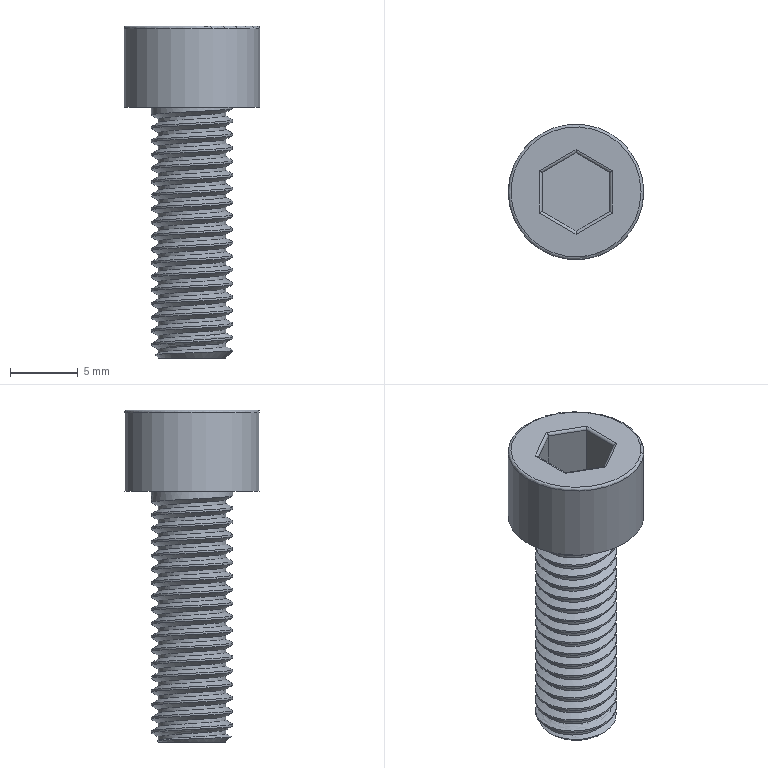Part | STEP file | Tube feed_id1810_x_t | 1 solid | 26 faces | box 10 x 10 x 24.5 mm | volume 797.459 mm3 | plane 12 | cylinder 9 | spline 3 | cone 1 | torus 1 | commonest cylinder face diameters 0.4 x6 5 x1 6 x1 10 x1